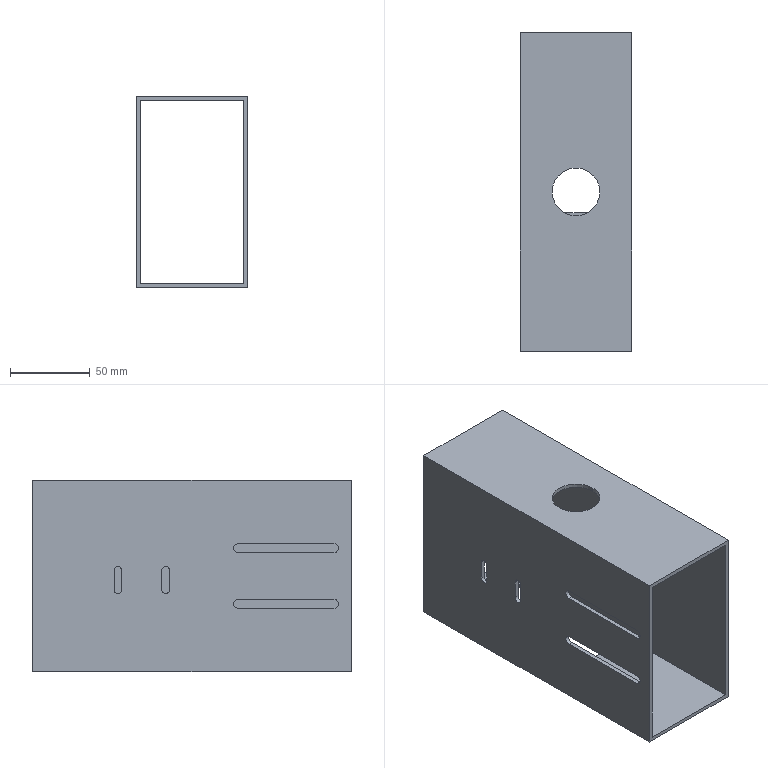Part | SolidWorks | features HoleWzd 2, Cut 1, Extrusion 1, ICE 1 | 1 solid | 34 faces | box 70 x 200 x 120 mm | volume 169957 mm3 | plane 22 | cylinder 12 | commonest cylinder face diameters 4.8 x6 5.8 x4 30 x2
STEP:
#1=CARTESIAN_POINT('',(2.5,48.9,-56.5));
#2=VERTEX_POINT('',#1);
#3=CARTESIAN_POINT('',(2.5,46.5,-54.1));
#4=VERTEX_POINT('',#3);
#5=CARTESIAN_POINT('',(2.5,46.5,-56.5));
#6=DIRECTION('',(1.,0.,0.));
#7=DIRECTION('',(0.,0.,-1.));
#8=AXIS2_PLACEMENT_3D('',#5,#6,#7);
#9=CIRCLE('',#8,2.4);
#10=EDGE_CURVE('',#2,#4,#9,.T.);
#11=ORIENTED_EDGE('',*,*,#10,.T.);
#12=CARTESIAN_POINT('',(0.,46.5,-54.1));
#13=VERTEX_POINT('',#12);
#14=CARTESIAN_POINT('',(0.,46.5,-54.1));
#15=DIRECTION('',(-1.,0.,0.));
#16=VECTOR('',#15,1000.);
#17=LINE('',#14,#16);
#18=EDGE_CURVE('',#4,#13,#17,.T.);
#19=ORIENTED_EDGE('',*,*,#18,.T.);
#20=CARTESIAN_POINT('',(0.,48.9,-56.5));
#21=VERTEX_POINT('',#20);
#22=CARTESIAN_POINT('',(0.,46.5,-56.5));
#23=DIRECTION('',(-1.,0.,0.));
#24=DIRECTION('',(0.,0.,1.));
#25=AXIS2_PLACEMENT_3D('',#22,#23,#24);
#26=CIRCLE('',#25,2.4);
#27=EDGE_CURVE('',#13,#21,#26,.T.);
#28=ORIENTED_EDGE('',*,*,#27,.T.);
#29=CARTESIAN_POINT('',(2.501,48.9,-56.5));
#30=DIRECTION('',(1.,0.,0.));
#31=VECTOR('',#30,1000.);
#32=LINE('',#29,#31);
#33=EDGE_CURVE('',#21,#2,#32,.T.);
#34=ORIENTED_EDGE('',*,*,#33,.T.);
#35=EDGE_LOOP('',(#11,#19,#28,#34));
#36=FACE_OUTER_BOUND('',#35,.T.);
#37=CARTESIAN_POINT('',(0.,46.5,-56.5));
#38=DIRECTION('',(-1.,0.,0.));
#39=DIRECTION('',(0.,0.,1.));
#40=AXIS2_PLACEMENT_3D('',#37,#38,#39);
#41=CYLINDRICAL_SURFACE('',#40,2.4);
#42=ADVANCED_FACE('',(#36),#41,.F.);
#43=CARTESIAN_POINT('',(2.5,18.9,-56.5));
#44=VERTEX_POINT('',#43);
#45=CARTESIAN_POINT('',(2.5,16.5,-54.1));
#46=VERTEX_POINT('',#45);
#47=CARTESIAN_POINT('',(2.5,16.5,-56.5));
#48=DIRECTION('',(1.,0.,0.));
#49=DIRECTION('',(0.,0.,-1.));
#50=AXIS2_PLACEMENT_3D('',#47,#48,#49);
#51=CIRCLE('',#50,2.4);
#52=EDGE_CURVE('',#44,#46,#51,.T.);
#53=ORIENTED_EDGE('',*,*,#52,.T.);
#54=CARTESIAN_POINT('',(0.,16.5,-54.1));
#55=VERTEX_POINT('',#54);
#56=CARTESIAN_POINT('',(0.,16.5,-54.1));
#57=DIRECTION('',(-1.,0.,0.));
#58=VECTOR('',#57,1000.);
#59=LINE('',#56,#58);
#60=EDGE_CURVE('',#46,#55,#59,.T.);
#61=ORIENTED_EDGE('',*,*,#60,.T.);
#62=CARTESIAN_POINT('',(0.,18.9,-56.5));
#63=VERTEX_POINT('',#62);
#64=CARTESIAN_POINT('',(0.,16.5,-56.5));
#65=DIRECTION('',(-1.,0.,0.));
#66=DIRECTION('',(0.,0.,1.));
#67=AXIS2_PLACEMENT_3D('',#64,#65,#66);
#68=CIRCLE('',#67,2.4);
#69=EDGE_CURVE('',#55,#63,#68,.T.);
#70=ORIENTED_EDGE('',*,*,#69,.T.);
#71=CARTESIAN_POINT('',(2.501,18.9,-56.5));
#72=DIRECTION('',(1.,0.,0.));
#73=VECTOR('',#72,1000.);
#74=LINE('',#71,#73);
#75=EDGE_CURVE('',#63,#44,#74,.T.);
#76=ORIENTED_EDGE('',*,*,#75,.T.);
#77=EDGE_LOOP('',(#53,#61,#70,#76));
#78=FACE_OUTER_BOUND('',#77,.T.);
#79=CARTESIAN_POINT('',(0.,16.5,-56.5));
#80=DIRECTION('',(-1.,0.,0.));
#81=DIRECTION('',(0.,0.,1.));
#82=AXIS2_PLACEMENT_3D('',#79,#80,#81);
#83=CYLINDRICAL_SURFACE('',#82,2.4);
#84=ADVANCED_FACE('',(#78),#83,.F.);
#85=CARTESIAN_POINT('',(20.,0.,-2.5));
#86=VERTEX_POINT('',#85);
#87=CARTESIAN_POINT('',(50.,0.,-2.5));
#88=VERTEX_POINT('',#87);
#89=CARTESIAN_POINT('',(35.,0.,-2.5));
#90=DIRECTION('',(0.,0.,1.));
#91=DIRECTION('',(-1.,0.,0.));
#92=AXIS2_PLACEMENT_3D('',#89,#90,#91);
#93=CIRCLE('',#92,15.);
#94=EDGE_CURVE('',#86,#88,#93,.T.);
#95=ORIENTED_EDGE('',*,*,#94,.F.);
#96=CARTESIAN_POINT('',(20.,0.,0.));
#97=VERTEX_POINT('',#96);
#98=CARTESIAN_POINT('',(20.,0.,-120.001));
#99=DIRECTION('',(0.,0.,1.));
#100=VECTOR('',#99,1000.);
#101=LINE('',#98,#100);
#102=EDGE_CURVE('',#86,#97,#101,.T.);
#103=ORIENTED_EDGE('',*,*,#102,.T.);
#104=CARTESIAN_POINT('',(50.,0.,0.));
#105=VERTEX_POINT('',#104);
#106=CARTESIAN_POINT('',(35.,0.,0.));
#107=DIRECTION('',(0.,0.,1.));
#108=DIRECTION('',(1.,0.,0.));
#109=AXIS2_PLACEMENT_3D('',#106,#107,#108);
#110=CIRCLE('',#109,15.);
#111=EDGE_CURVE('',#97,#105,#110,.T.);
#112=ORIENTED_EDGE('',*,*,#111,.T.);
#113=CARTESIAN_POINT('',(50.,0.,-120.001));
#114=DIRECTION('',(0.,0.,1.));
#115=VECTOR('',#114,1000.);
#116=LINE('',#113,#115);
#117=EDGE_CURVE('',#88,#105,#116,.T.);
#118=ORIENTED_EDGE('',*,*,#117,.F.);
#119=EDGE_LOOP('',(#95,#103,#112,#118));
#120=FACE_OUTER_BOUND('',#119,.T.);
#121=CARTESIAN_POINT('',(35.,0.,-120.001));
#122=DIRECTION('',(0.,0.,1.));
#123=DIRECTION('',(1.,0.,0.));
#124=AXIS2_PLACEMENT_3D('',#121,#122,#123);
#125=CYLINDRICAL_SURFACE('',#124,15.);
#126=ADVANCED_FACE('',(#120),#125,.F.);
#127=CARTESIAN_POINT('',(0.,-89.,-39.6));
#128=VERTEX_POINT('',#127);
#129=CARTESIAN_POINT('',(0.,-29.,-39.6));
#130=VERTEX_POINT('',#129);
#131=CARTESIAN_POINT('',(0.,-89.,-39.6));
#132=DIRECTION('',(0.,1.,0.));
#133=VECTOR('',#132,1000.);
#134=LINE('',#131,#133);
#135=EDGE_CURVE('',#128,#130,#134,.T.);
#136=ORIENTED_EDGE('',*,*,#135,.F.);
#137=CARTESIAN_POINT('',(0.,-89.,-45.4));
#138=VERTEX_POINT('',#137);
#139=CARTESIAN_POINT('',(0.,-89.,-42.5));
#140=DIRECTION('',(-1.,0.,0.));
#141=DIRECTION('',(0.,0.,1.));
#142=AXIS2_PLACEMENT_3D('',#139,#140,#141);
#143=CIRCLE('',#142,2.9);
#144=EDGE_CURVE('',#138,#128,#143,.T.);
#145=ORIENTED_EDGE('',*,*,#144,.F.);
#146=CARTESIAN_POINT('',(0.,-29.,-45.4));
#147=VERTEX_POINT('',#146);
#148=CARTESIAN_POINT('',(0.,-89.,-45.4));
#149=DIRECTION('',(0.,1.,0.));
#150=VECTOR('',#149,1000.);
#151=LINE('',#148,#150);
#152=EDGE_CURVE('',#138,#147,#151,.T.);
#153=ORIENTED_EDGE('',*,*,#152,.T.);
#154=CARTESIAN_POINT('',(0.,-29.,-42.5));
#155=DIRECTION('',(-1.,0.,0.));
#156=DIRECTION('',(0.,0.,1.));
#157=AXIS2_PLACEMENT_3D('',#154,#155,#156);
#158=CIRCLE('',#157,2.9);
#159=EDGE_CURVE('',#130,#147,#158,.T.);
#160=ORIENTED_EDGE('',*,*,#159,.F.);
#161=EDGE_LOOP('',(#136,#145,#153,#160));
#162=FACE_BOUND('',#161,.T.);
#163=CARTESIAN_POINT('',(0.,48.9,-68.5));
#164=VERTEX_POINT('',#163);
#165=CARTESIAN_POINT('',(0.,48.9,-68.5));
#166=DIRECTION('',(0.,0.,1.));
#167=VECTOR('',#166,1000.);
#168=LINE('',#165,#167);
#169=EDGE_CURVE('',#164,#21,#168,.T.);
#170=ORIENTED_EDGE('',*,*,#169,.T.);
#171=ORIENTED_EDGE('',*,*,#27,.F.);
#172=CARTESIAN_POINT('',(0.,44.1,-56.5));
#173=VERTEX_POINT('',#172);
#174=CARTESIAN_POINT('',(0.,46.5,-56.5));
#175=DIRECTION('',(-1.,0.,0.));
#176=DIRECTION('',(0.,0.,1.));
#177=AXIS2_PLACEMENT_3D('',#174,#175,#176);
#178=CIRCLE('',#177,2.4);
#179=EDGE_CURVE('',#173,#13,#178,.T.);
#180=ORIENTED_EDGE('',*,*,#179,.F.);
#181=CARTESIAN_POINT('',(0.,44.1,-68.5));
#182=VERTEX_POINT('',#181);
#183=CARTESIAN_POINT('',(0.,44.1,-68.5));
#184=DIRECTION('',(0.,0.,1.));
#185=VECTOR('',#184,1000.);
#186=LINE('',#183,#185);
#187=EDGE_CURVE('',#182,#173,#186,.T.);
#188=ORIENTED_EDGE('',*,*,#187,.F.);
#189=CARTESIAN_POINT('',(0.,46.5,-68.5));
#190=DIRECTION('',(-1.,0.,0.));
#191=DIRECTION('',(0.,0.,1.));
#192=AXIS2_PLACEMENT_3D('',#189,#190,#191);
#193=CIRCLE('',#192,2.4);
#194=EDGE_CURVE('',#164,#182,#193,.T.);
#195=ORIENTED_EDGE('',*,*,#194,.F.);
#196=EDGE_LOOP('',(#170,#171,#180,#188,#195));
#197=FACE_BOUND('',#196,.T.);
#198=CARTESIAN_POINT('',(0.,-100.,-120.));
#199=VERTEX_POINT('',#198);
#200=CARTESIAN_POINT('',(0.,-100.,0.));
#201=VERTEX_POINT('',#200);
#202=CARTESIAN_POINT('',(0.,-100.,0.));
#203=DIRECTION('',(0.,0.,1.));
#204=VECTOR('',#203,1000.);
#205=LINE('',#202,#204);
#206=EDGE_CURVE('',#199,#201,#205,.T.);
#207=ORIENTED_EDGE('',*,*,#206,.T.);
#208=CARTESIAN_POINT('',(0.,100.,0.));
#209=VERTEX_POINT('',#208);
#210=CARTESIAN_POINT('',(0.,100.,0.));
#211=DIRECTION('',(0.,-1.,0.));
#212=VECTOR('',#211,1000.);
#213=LINE('',#210,#212);
#214=EDGE_CURVE('',#209,#201,#213,.T.);
#215=ORIENTED_EDGE('',*,*,#214,.F.);
#216=CARTESIAN_POINT('',(0.,100.,-120.));
#217=VERTEX_POINT('',#216);
#218=CARTESIAN_POINT('',(0.,100.,0.));
#219=DIRECTION('',(0.,0.,1.));
#220=VECTOR('',#219,1000.);
#221=LINE('',#218,#220);
#222=EDGE_CURVE('',#217,#209,#221,.T.);
#223=ORIENTED_EDGE('',*,*,#222,.F.);
#224=CARTESIAN_POINT('',(0.,100.,-120.));
#225=DIRECTION('',(0.,-1.,0.));
#226=VECTOR('',#225,1000.);
#227=LINE('',#224,#226);
#228=EDGE_CURVE('',#217,#199,#227,.T.);
#229=ORIENTED_EDGE('',*,*,#228,.T.);
#230=EDGE_LOOP('',(#207,#215,#223,#229));
#231=FACE_OUTER_BOUND('',#230,.T.);
#232=CARTESIAN_POINT('',(0.,14.1,-56.5));
#233=VERTEX_POINT('',#232);
#234=CARTESIAN_POINT('',(0.,16.5,-56.5));
#235=DIRECTION('',(-1.,0.,0.));
#236=DIRECTION('',(0.,0.,1.));
#237=AXIS2_PLACEMENT_3D('',#234,#235,#236);
#238=CIRCLE('',#237,2.4);
#239=EDGE_CURVE('',#233,#55,#238,.T.);
#240=ORIENTED_EDGE('',*,*,#239,.F.);
#241=CARTESIAN_POINT('',(0.,14.1,-68.5));
#242=VERTEX_POINT('',#241);
#243=CARTESIAN_POINT('',(0.,14.1,-68.5));
#244=DIRECTION('',(0.,0.,1.));
#245=VECTOR('',#244,1000.);
#246=LINE('',#243,#245);
#247=EDGE_CURVE('',#242,#233,#246,.T.);
#248=ORIENTED_EDGE('',*,*,#247,.F.);
#249=CARTESIAN_POINT('',(0.,18.9,-68.5));
#250=VERTEX_POINT('',#249);
#251=CARTESIAN_POINT('',(0.,16.5,-68.5));
#252=DIRECTION('',(-1.,0.,0.));
#253=DIRECTION('',(0.,0.,1.));
#254=AXIS2_PLACEMENT_3D('',#251,#252,#253);
#255=CIRCLE('',#254,2.4);
#256=EDGE_CURVE('',#250,#242,#255,.T.);
#257=ORIENTED_EDGE('',*,*,#256,.F.);
#258=CARTESIAN_POINT('',(0.,18.9,-68.5));
#259=DIRECTION('',(0.,0.,1.));
#260=VECTOR('',#259,1000.);
#261=LINE('',#258,#260);
#262=EDGE_CURVE('',#250,#63,#261,.T.);
#263=ORIENTED_EDGE('',*,*,#262,.T.);
#264=ORIENTED_EDGE('',*,*,#69,.F.);
#265=EDGE_LOOP('',(#240,#248,#257,#263,#264));
#266=FACE_BOUND('',#265,.T.);
#267=CARTESIAN_POINT('',(0.,-89.,-74.6));
#268=VERTEX_POINT('',#267);
#269=CARTESIAN_POINT('',(0.,-29.,-74.6));
#270=VERTEX_POINT('',#269);
#271=CARTESIAN_POINT('',(0.,-89.,-74.6));
#272=DIRECTION('',(0.,1.,0.));
#273=VECTOR('',#272,1000.);
#274=LINE('',#271,#273);
#275=EDGE_CURVE('',#268,#270,#274,.T.);
#276=ORIENTED_EDGE('',*,*,#275,.F.);
#277=CARTESIAN_POINT('',(0.,-89.,-80.4));
#278=VERTEX_POINT('',#277);
#279=CARTESIAN_POINT('',(0.,-89.,-77.5));
#280=DIRECTION('',(-1.,0.,0.));
#281=DIRECTION('',(0.,0.,1.));
#282=AXIS2_PLACEMENT_3D('',#279,#280,#281);
#283=CIRCLE('',#282,2.9);
#284=EDGE_CURVE('',#278,#268,#283,.T.);
#285=ORIENTED_EDGE('',*,*,#284,.F.);
#286=CARTESIAN_POINT('',(0.,-29.,-80.4));
#287=VERTEX_POINT('',#286);
#288=CARTESIAN_POINT('',(0.,-89.,-80.4));
#289=DIRECTION('',(0.,1.,0.));
#290=VECTOR('',#289,1000.);
#291=LINE('',#288,#290);
#292=EDGE_CURVE('',#278,#287,#291,.T.);
#293=ORIENTED_EDGE('',*,*,#292,.T.);
#294=CARTESIAN_POINT('',(0.,-29.,-77.5));
#295=DIRECTION('',(-1.,0.,0.));
#296=DIRECTION('',(0.,0.,1.));
#297=AXIS2_PLACEMENT_3D('',#294,#295,#296);
#298=CIRCLE('',#297,2.9);
#299=EDGE_CURVE('',#270,#287,#298,.T.);
#300=ORIENTED_EDGE('',*,*,#299,.F.);
#301=EDGE_LOOP('',(#276,#285,#293,#300));
#302=FACE_BOUND('',#301,.T.);
#303=CARTESIAN_POINT('',(0.,100.,0.));
#304=DIRECTION('',(1.,0.,0.));
#305=DIRECTION('',(0.,0.,-1.));
#306=AXIS2_PLACEMENT_3D('',#303,#304,#305);
#307=PLANE('',#306);
#308=ADVANCED_FACE('',(#162,#197,#231,#266,#302),#307,.F.);
#309=CARTESIAN_POINT('',(2.5,-89.,-80.4));
#310=VERTEX_POINT('',#309);
#311=CARTESIAN_POINT('',(2.5,-29.,-80.4));
#312=VERTEX_POINT('',#311);
#313=CARTESIAN_POINT('',(2.5,100.,-80.4));
#314=DIRECTION('',(0.,1.,0.));
#315=VECTOR('',#314,1000.);
#316=LINE('',#313,#315);
#317=EDGE_CURVE('',#310,#312,#316,.T.);
#318=ORIENTED_EDGE('',*,*,#317,.F.);
#319=CARTESIAN_POINT('',(2.5,-89.,-74.6));
#320=VERTEX_POINT('',#319);
#321=CARTESIAN_POINT('',(2.5,-89.,-77.5));
#322=DIRECTION('',(1.,0.,0.));
#323=DIRECTION('',(0.,0.,-1.));
#324=AXIS2_PLACEMENT_3D('',#321,#322,#323);
#325=CIRCLE('',#324,2.9);
#326=EDGE_CURVE('',#320,#310,#325,.T.);
#327=ORIENTED_EDGE('',*,*,#326,.F.);
#328=CARTESIAN_POINT('',(2.5,-29.,-74.6));
#329=VERTEX_POINT('',#328);
#330=CARTESIAN_POINT('',(2.5,100.,-74.6));
#331=DIRECTION('',(0.,-1.,0.));
#332=VECTOR('',#331,1000.);
#333=LINE('',#330,#332);
#334=EDGE_CURVE('',#329,#320,#333,.T.);
#335=ORIENTED_EDGE('',*,*,#334,.F.);
#336=CARTESIAN_POINT('',(2.5,-29.,-77.5));
#337=DIRECTION('',(1.,0.,0.));
#338=DIRECTION('',(0.,0.,-1.));
#339=AXIS2_PLACEMENT_3D('',#336,#337,#338);
#340=CIRCLE('',#339,2.9);
#341=EDGE_CURVE('',#312,#329,#340,.T.);
#342=ORIENTED_EDGE('',*,*,#341,.F.);
#343=EDGE_LOOP('',(#318,#327,#335,#342));
#344=FACE_BOUND('',#343,.T.);
#345=CARTESIAN_POINT('',(2.5,-89.,-45.4));
#346=VERTEX_POINT('',#345);
#347=CARTESIAN_POINT('',(2.5,-29.,-45.4));
#348=VERTEX_POINT('',#347);
#349=CARTESIAN_POINT('',(2.5,100.,-45.4));
#350=DIRECTION('',(0.,1.,0.));
#351=VECTOR('',#350,1000.);
#352=LINE('',#349,#351);
#353=EDGE_CURVE('',#346,#348,#352,.T.);
#354=ORIENTED_EDGE('',*,*,#353,.F.);
#355=CARTESIAN_POINT('',(2.5,-89.,-39.6));
#356=VERTEX_POINT('',#355);
#357=CARTESIAN_POINT('',(2.5,-89.,-42.5));
#358=DIRECTION('',(1.,0.,0.));
#359=DIRECTION('',(0.,0.,-1.));
#360=AXIS2_PLACEMENT_3D('',#357,#358,#359);
#361=CIRCLE('',#360,2.9);
#362=EDGE_CURVE('',#356,#346,#361,.T.);
#363=ORIENTED_EDGE('',*,*,#362,.F.);
#364=CARTESIAN_POINT('',(2.5,-29.,-39.6));
#365=VERTEX_POINT('',#364);
#366=CARTESIAN_POINT('',(2.5,100.,-39.6));
#367=DIRECTION('',(0.,-1.,0.));
#368=VECTOR('',#367,1000.);
#369=LINE('',#366,#368);
#370=EDGE_CURVE('',#365,#356,#369,.T.);
#371=ORIENTED_EDGE('',*,*,#370,.F.);
#372=CARTESIAN_POINT('',(2.5,-29.,-42.5));
#373=DIRECTION('',(1.,0.,0.));
#374=DIRECTION('',(0.,0.,-1.));
#375=AXIS2_PLACEMENT_3D('',#372,#373,#374);
#376=CIRCLE('',#375,2.9);
#377=EDGE_CURVE('',#348,#365,#376,.T.);
#378=ORIENTED_EDGE('',*,*,#377,.F.);
#379=EDGE_LOOP('',(#354,#363,#371,#378));
#380=FACE_BOUND('',#379,.T.);
#381=CARTESIAN_POINT('',(2.5,-100.,-117.5));
#382=VERTEX_POINT('',#381);
#383=CARTESIAN_POINT('',(2.5,-100.,-2.5));
#384=VERTEX_POINT('',#383);
#385=CARTESIAN_POINT('',(2.5,-100.,-2.5));
#386=DIRECTION('',(0.,0.,1.));
#387=VECTOR('',#386,1000.);
#388=LINE('',#385,#387);
#389=EDGE_CURVE('',#382,#384,#388,.T.);
#390=ORIENTED_EDGE('',*,*,#389,.F.);
#391=CARTESIAN_POINT('',(2.5,100.,-117.5));
#392=VERTEX_POINT('',#391);
#393=CARTESIAN_POINT('',(2.5,100.,-117.5));
#394=DIRECTION('',(0.,-1.,0.));
#395=VECTOR('',#394,1000.);
#396=LINE('',#393,#395);
#397=EDGE_CURVE('',#392,#382,#396,.T.);
#398=ORIENTED_EDGE('',*,*,#397,.F.);
#399=CARTESIAN_POINT('',(2.5,100.,-2.5));
#400=VERTEX_POINT('',#399);
#401=CARTESIAN_POINT('',(2.5,100.,-2.5));
#402=DIRECTION('',(0.,0.,1.));
#403=VECTOR('',#402,1000.);
#404=LINE('',#401,#403);
#405=EDGE_CURVE('',#392,#400,#404,.T.);
#406=ORIENTED_EDGE('',*,*,#405,.T.);
#407=CARTESIAN_POINT('',(2.5,100.,-2.5));
#408=DIRECTION('',(0.,-1.,0.));
#409=VECTOR('',#408,1000.);
#410=LINE('',#407,#409);
#411=EDGE_CURVE('',#400,#384,#410,.T.);
#412=ORIENTED_EDGE('',*,*,#411,.T.);
#413=EDGE_LOOP('',(#390,#398,#406,#412));
#414=FACE_OUTER_BOUND('',#413,.T.);
#415=ORIENTED_EDGE('',*,*,#52,.F.);
#416=CARTESIAN_POINT('',(2.5,18.9,-68.5));
#417=VERTEX_POINT('',#416);
#418=CARTESIAN_POINT('',(2.5,18.9,-2.5));
#419=DIRECTION('',(0.,0.,-1.));
#420=VECTOR('',#419,1000.);
#421=LINE('',#418,#420);
#422=EDGE_CURVE('',#44,#417,#421,.T.);
#423=ORIENTED_EDGE('',*,*,#422,.T.);
#424=CARTESIAN_POINT('',(2.5,14.1,-68.5));
#425=VERTEX_POINT('',#424);
#426=CARTESIAN_POINT('',(2.5,16.5,-68.5));
#427=DIRECTION('',(1.,0.,0.));
#428=DIRECTION('',(0.,0.,-1.));
#429=AXIS2_PLACEMENT_3D('',#426,#427,#428);
#430=CIRCLE('',#429,2.4);
#431=EDGE_CURVE('',#425,#417,#430,.T.);
#432=ORIENTED_EDGE('',*,*,#431,.F.);
#433=CARTESIAN_POINT('',(2.5,14.1,-56.5));
#434=VERTEX_POINT('',#433);
#435=CARTESIAN_POINT('',(2.5,14.1,-2.5));
#436=DIRECTION('',(0.,0.,-1.));
#437=VECTOR('',#436,1000.);
#438=LINE('',#435,#437);
#439=EDGE_CURVE('',#434,#425,#438,.T.);
#440=ORIENTED_EDGE('',*,*,#439,.F.);
#441=CARTESIAN_POINT('',(2.5,16.5,-56.5));
#442=DIRECTION('',(1.,0.,0.));
#443=DIRECTION('',(0.,0.,-1.));
#444=AXIS2_PLACEMENT_3D('',#441,#442,#443);
#445=CIRCLE('',#444,2.4);
#446=EDGE_CURVE('',#46,#434,#445,.T.);
#447=ORIENTED_EDGE('',*,*,#446,.F.);
#448=EDGE_LOOP('',(#415,#423,#432,#440,#447));
#449=FACE_BOUND('',#448,.T.);
#450=ORIENTED_EDGE('',*,*,#10,.F.);
#451=CARTESIAN_POINT('',(2.5,48.9,-68.5));
#452=VERTEX_POINT('',#451);
#453=CARTESIAN_POINT('',(2.5,48.9,-2.5));
#454=DIRECTION('',(0.,0.,-1.));
#455=VECTOR('',#454,1000.);
#456=LINE('',#453,#455);
#457=EDGE_CURVE('',#2,#452,#456,.T.);
#458=ORIENTED_EDGE('',*,*,#457,.T.);
#459=CARTESIAN_POINT('',(2.5,44.1,-68.5));
#460=VERTEX_POINT('',#459);
#461=CARTESIAN_POINT('',(2.5,46.5,-68.5));
#462=DIRECTION('',(1.,0.,0.));
#463=DIRECTION('',(0.,0.,-1.));
#464=AXIS2_PLACEMENT_3D('',#461,#462,#463);
#465=CIRCLE('',#464,2.4);
#466=EDGE_CURVE('',#460,#452,#465,.T.);
#467=ORIENTED_EDGE('',*,*,#466,.F.);
#468=CARTESIAN_POINT('',(2.5,44.1,-56.5));
#469=VERTEX_POINT('',#468);
#470=CARTESIAN_POINT('',(2.5,44.1,-2.5));
#471=DIRECTION('',(0.,0.,-1.));
#472=VECTOR('',#471,1000.);
#473=LINE('',#470,#472);
#474=EDGE_CURVE('',#469,#460,#473,.T.);
#475=ORIENTED_EDGE('',*,*,#474,.F.);
#476=CARTESIAN_POINT('',(2.5,46.5,-56.5));
#477=DIRECTION('',(1.,0.,0.));
#478=DIRECTION('',(0.,0.,-1.));
#479=AXIS2_PLACEMENT_3D('',#476,#477,#478);
#480=CIRCLE('',#479,2.4);
#481=EDGE_CURVE('',#4,#469,#480,.T.);
#482=ORIENTED_EDGE('',*,*,#481,.F.);
#483=EDGE_LOOP('',(#450,#458,#467,#475,#482));
#484=FACE_BOUND('',#483,.T.);
#485=CARTESIAN_POINT('',(2.5,100.,-2.5));
#486=DIRECTION('',(1.,0.,0.));
#487=DIRECTION('',(0.,0.,-1.));
#488=AXIS2_PLACEMENT_3D('',#485,#486,#487);
#489=PLANE('',#488);
#490=ADVANCED_FACE('',(#344,#380,#414,#449,#484),#489,.T.);
#491=ORIENTED_EDGE('',*,*,#222,.T.);
#492=CARTESIAN_POINT('',(70.,100.,0.));
#493=VERTEX_POINT('',#492);
#494=CARTESIAN_POINT('',(0.,100.,0.));
#495=DIRECTION('',(1.,0.,0.));
#496=VECTOR('',#495,1000.);
#497=LINE('',#494,#496);
#498=EDGE_CURVE('',#209,#493,#497,.T.);
#499=ORIENTED_EDGE('',*,*,#498,.T.);
#500=CARTESIAN_POINT('',(70.,100.,-120.));
#501=VERTEX_POINT('',#500);
#502=CARTESIAN_POINT('',(70.,100.,0.));
#503=DIRECTION('',(0.,0.,-1.));
#504=VECTOR('',#503,1000.);
#505=LINE('',#502,#504);
#506=EDGE_CURVE('',#493,#501,#505,.T.);
#507=ORIENTED_EDGE('',*,*,#506,.T.);
#508=CARTESIAN_POINT('',(0.,100.,-120.));
#509=DIRECTION('',(-1.,0.,0.));
#510=VECTOR('',#509,1000.);
#511=LINE('',#508,#510);
#512=EDGE_CURVE('',#501,#217,#511,.T.);
#513=ORIENTED_EDGE('',*,*,#512,.T.);
#514=EDGE_LOOP('',(#491,#499,#507,#513));
#515=FACE_OUTER_BOUND('',#514,.T.);
#516=ORIENTED_EDGE('',*,*,#405,.F.);
#517=CARTESIAN_POINT('',(67.5,100.,-117.5));
#518=VERTEX_POINT('',#517);
#519=CARTESIAN_POINT('',(2.5,100.,-117.5));
#520=DIRECTION('',(-1.,0.,0.));
#521=VECTOR('',#520,1000.);
#522=LINE('',#519,#521);
#523=EDGE_CURVE('',#518,#392,#522,.T.);
#524=ORIENTED_EDGE('',*,*,#523,.F.);
#525=CARTESIAN_POINT('',(67.5,100.,-2.5));
#526=VERTEX_POINT('',#525);
#527=CARTESIAN_POINT('',(67.5,100.,-2.5));
#528=DIRECTION('',(0.,0.,-1.));
#529=VECTOR('',#528,1000.);
#530=LINE('',#527,#529);
#531=EDGE_CURVE('',#526,#518,#530,.T.);
#532=ORIENTED_EDGE('',*,*,#531,.F.);
#533=CARTESIAN_POINT('',(2.5,100.,-2.5));
#534=DIRECTION('',(1.,0.,0.));
#535=VECTOR('',#534,1000.);
#536=LINE('',#533,#535);
#537=EDGE_CURVE('',#400,#526,#536,.T.);
#538=ORIENTED_EDGE('',*,*,#537,.F.);
#539=EDGE_LOOP('',(#516,#524,#532,#538));
#540=FACE_BOUND('',#539,.T.);
#541=CARTESIAN_POINT('',(0.,100.,0.));
#542=DIRECTION('',(0.,-1.,0.));
#543=DIRECTION('',(0.,0.,-1.));
#544=AXIS2_PLACEMENT_3D('',#541,#542,#543);
#545=PLANE('',#544);
#546=ADVANCED_FACE('',(#515,#540),#545,.F.);
#547=ORIENTED_EDGE('',*,*,#206,.F.);
#548=CARTESIAN_POINT('',(70.,-100.,-120.));
#549=VERTEX_POINT('',#548);
#550=CARTESIAN_POINT('',(0.,-100.,-120.));
#551=DIRECTION('',(-1.,0.,0.));
#552=VECTOR('',#551,1000.);
#553=LINE('',#550,#552);
#554=EDGE_CURVE('',#549,#199,#553,.T.);
#555=ORIENTED_EDGE('',*,*,#554,.F.);
#556=CARTESIAN_POINT('',(70.,-100.,0.));
#557=VERTEX_POINT('',#556);
#558=CARTESIAN_POINT('',(70.,-100.,0.));
#559=DIRECTION('',(0.,0.,-1.));
#560=VECTOR('',#559,1000.);
#561=LINE('',#558,#560);
#562=EDGE_CURVE('',#557,#549,#561,.T.);
#563=ORIENTED_EDGE('',*,*,#562,.F.);
#564=CARTESIAN_POINT('',(0.,-100.,0.));
#565=DIRECTION('',(1.,0.,0.));
#566=VECTOR('',#565,1000.);
#567=LINE('',#564,#566);
#568=EDGE_CURVE('',#201,#557,#567,.T.);
#569=ORIENTED_EDGE('',*,*,#568,.F.);
#570=EDGE_LOOP('',(#547,#555,#563,#569));
#571=FACE_OUTER_BOUND('',#570,.T.);
#572=CARTESIAN_POINT('',(67.5,-100.,-117.5));
#573=VERTEX_POINT('',#572);
#574=CARTESIAN_POINT('',(2.5,-100.,-117.5));
#575=DIRECTION('',(-1.,0.,0.));
#576=VECTOR('',#575,1000.);
#577=LINE('',#574,#576);
#578=EDGE_CURVE('',#573,#382,#577,.T.);
#579=ORIENTED_EDGE('',*,*,#578,.T.);
#580=ORIENTED_EDGE('',*,*,#389,.T.);
#581=CARTESIAN_POINT('',(67.5,-100.,-2.5));
#582=VERTEX_POINT('',#581);
#583=CARTESIAN_POINT('',(2.5,-100.,-2.5));
#584=DIRECTION('',(1.,0.,0.));
#585=VECTOR('',#584,1000.);
#586=LINE('',#583,#585);
#587=EDGE_CURVE('',#384,#582,#586,.T.);
#588=ORIENTED_EDGE('',*,*,#587,.T.);
#589=CARTESIAN_POINT('',(67.5,-100.,-2.5));
#590=DIRECTION('',(0.,0.,-1.));
#591=VECTOR('',#590,1000.);
#592=LINE('',#589,#591);
#593=EDGE_CURVE('',#582,#573,#592,.T.);
#594=ORIENTED_EDGE('',*,*,#593,.T.);
#595=EDGE_LOOP('',(#579,#580,#588,#594));
#596=FACE_BOUND('',#595,.T.);
#597=CARTESIAN_POINT('',(0.,-100.,0.));
#598=DIRECTION('',(0.,-1.,0.));
#599=DIRECTION('',(0.,0.,-1.));
#600=AXIS2_PLACEMENT_3D('',#597,#598,#599);
#601=PLANE('',#600);
#602=ADVANCED_FACE('',(#571,#596),#601,.T.);
#603=CARTESIAN_POINT('',(35.,0.,0.));
#604=DIRECTION('',(0.,0.,1.));
#605=DIRECTION('',(1.,0.,0.));
#606=AXIS2_PLACEMENT_3D('',#603,#604,#605);
#607=CIRCLE('',#606,15.);
#608=EDGE_CURVE('',#105,#97,#607,.T.);
#609=ORIENTED_EDGE('',*,*,#608,.F.);
#610=ORIENTED_EDGE('',*,*,#111,.F.);
#611=EDGE_LOOP('',(#609,#610));
#612=FACE_BOUND('',#611,.T.);
#613=ORIENTED_EDGE('',*,*,#568,.T.);
#614=CARTESIAN_POINT('',(70.,100.,0.));
#615=DIRECTION('',(0.,-1.,0.));
#616=VECTOR('',#615,1000.);
#617=LINE('',#614,#616);
#618=EDGE_CURVE('',#493,#557,#617,.T.);
#619=ORIENTED_EDGE('',*,*,#618,.F.);
#620=ORIENTED_EDGE('',*,*,#498,.F.);
#621=ORIENTED_EDGE('',*,*,#214,.T.);
#622=EDGE_LOOP('',(#613,#619,#620,#621));
#623=FACE_OUTER_BOUND('',#622,.T.);
#624=CARTESIAN_POINT('',(0.,100.,0.));
#625=DIRECTION('',(0.,0.,-1.));
#626=DIRECTION('',(-1.,0.,0.));
#627=AXIS2_PLACEMENT_3D('',#624,#625,#626);
#628=PLANE('',#627);
#629=ADVANCED_FACE('',(#612,#623),#628,.F.);
#630=ORIENTED_EDGE('',*,*,#562,.T.);
#631=CARTESIAN_POINT('',(70.,100.,-120.));
#632=DIRECTION('',(0.,-1.,0.));
#633=VECTOR('',#632,1000.);
#634=LINE('',#631,#633);
#635=EDGE_CURVE('',#501,#549,#634,.T.);
#636=ORIENTED_EDGE('',*,*,#635,.F.);
#637=ORIENTED_EDGE('',*,*,#506,.F.);
#638=ORIENTED_EDGE('',*,*,#618,.T.);
#639=EDGE_LOOP('',(#630,#636,#637,#638));
#640=FACE_OUTER_BOUND('',#639,.T.);
#641=CARTESIAN_POINT('',(70.,100.,0.));
#642=DIRECTION('',(-1.,0.,0.));
#643=DIRECTION('',(0.,0.,1.));
#644=AXIS2_PLACEMENT_3D('',#641,#642,#643);
#645=PLANE('',#644);
#646=ADVANCED_FACE('',(#640),#645,.F.);
#647=CARTESIAN_POINT('',(61.,85.,-120.));
#648=VERTEX_POINT('',#647);
#649=CARTESIAN_POINT('',(61.,-13.,-120.));
#650=VERTEX_POINT('',#649);
#651=CARTESIAN_POINT('',(61.,-13.,-120.));
#652=DIRECTION('',(0.,-1.,0.));
#653=VECTOR('',#652,1000.);
#654=LINE('',#651,#653);
#655=EDGE_CURVE('',#648,#650,#654,.T.);
#656=ORIENTED_EDGE('',*,*,#655,.F.);
#657=CARTESIAN_POINT('',(16.,85.,-120.));
#658=VERTEX_POINT('',#657);
#659=CARTESIAN_POINT('',(61.,85.,-120.));
#660=DIRECTION('',(1.,0.,0.));
#661=VECTOR('',#660,1000.);
#662=LINE('',#659,#661);
#663=EDGE_CURVE('',#658,#648,#662,.T.);
#664=ORIENTED_EDGE('',*,*,#663,.F.);
#665=CARTESIAN_POINT('',(16.,-13.,-120.));
#666=VERTEX_POINT('',#665);
#667=CARTESIAN_POINT('',(16.,-13.,-120.));
#668=DIRECTION('',(0.,1.,0.));
#669=VECTOR('',#668,1000.);
#670=LINE('',#667,#669);
#671=EDGE_CURVE('',#666,#658,#670,.T.);
#672=ORIENTED_EDGE('',*,*,#671,.F.);
#673=CARTESIAN_POINT('',(61.,-13.,-120.));
#674=DIRECTION('',(-1.,0.,0.));
#675=VECTOR('',#674,1000.);
#676=LINE('',#673,#675);
#677=EDGE_CURVE('',#650,#666,#676,.T.);
#678=ORIENTED_EDGE('',*,*,#677,.F.);
#679=EDGE_LOOP('',(#656,#664,#672,#678));
#680=FACE_BOUND('',#679,.T.);
#681=ORIENTED_EDGE('',*,*,#554,.T.);
#682=ORIENTED_EDGE('',*,*,#228,.F.);
#683=ORIENTED_EDGE('',*,*,#512,.F.);
#684=ORIENTED_EDGE('',*,*,#635,.T.);
#685=EDGE_LOOP('',(#681,#682,#683,#684));
#686=FACE_OUTER_BOUND('',#685,.T.);
#687=CARTESIAN_POINT('',(0.,100.,-120.));
#688=DIRECTION('',(0.,0.,1.));
#689=DIRECTION('',(1.,0.,0.));
#690=AXIS2_PLACEMENT_3D('',#687,#688,#689);
#691=PLANE('',#690);
#692=ADVANCED_FACE('',(#680,#686),#691,.F.);
#693=CARTESIAN_POINT('',(35.,0.,-2.5));
#694=DIRECTION('',(0.,0.,1.));
#695=DIRECTION('',(-1.,0.,0.));
#696=AXIS2_PLACEMENT_3D('',#693,#694,#695);
#697=CIRCLE('',#696,15.);
#698=EDGE_CURVE('',#88,#86,#697,.T.);
#699=ORIENTED_EDGE('',*,*,#698,.T.);
#700=ORIENTED_EDGE('',*,*,#94,.T.);
#701=EDGE_LOOP('',(#699,#700));
#702=FACE_BOUND('',#701,.T.);
#703=ORIENTED_EDGE('',*,*,#587,.F.);
#704=ORIENTED_EDGE('',*,*,#411,.F.);
#705=ORIENTED_EDGE('',*,*,#537,.T.);
#706=CARTESIAN_POINT('',(67.5,100.,-2.5));
#707=DIRECTION('',(0.,-1.,0.));
#708=VECTOR('',#707,1000.);
#709=LINE('',#706,#708);
#710=EDGE_CURVE('',#526,#582,#709,.T.);
#711=ORIENTED_EDGE('',*,*,#710,.T.);
#712=EDGE_LOOP('',(#703,#704,#705,#711));
#713=FACE_OUTER_BOUND('',#712,.T.);
#714=CARTESIAN_POINT('',(2.5,100.,-2.5));
#715=DIRECTION('',(0.,0.,-1.));
#716=DIRECTION('',(-1.,0.,0.));
#717=AXIS2_PLACEMENT_3D('',#714,#715,#716);
#718=PLANE('',#717);
#719=ADVANCED_FACE('',(#702,#713),#718,.T.);
#720=ORIENTED_EDGE('',*,*,#593,.F.);
#721=ORIENTED_EDGE('',*,*,#710,.F.);
#722=ORIENTED_EDGE('',*,*,#531,.T.);
#723=CARTESIAN_POINT('',(67.5,100.,-117.5));
#724=DIRECTION('',(0.,-1.,0.));
#725=VECTOR('',#724,1000.);
#726=LINE('',#723,#725);
#727=EDGE_CURVE('',#518,#573,#726,.T.);
#728=ORIENTED_EDGE('',*,*,#727,.T.);
#729=EDGE_LOOP('',(#720,#721,#722,#728));
#730=FACE_OUTER_BOUND('',#729,.T.);
#731=CARTESIAN_POINT('',(67.5,100.,-2.5));
#732=DIRECTION('',(-1.,0.,0.));
#733=DIRECTION('',(0.,0.,1.));
#734=AXIS2_PLACEMENT_3D('',#731,#732,#733);
#735=PLANE('',#734);
#736=ADVANCED_FACE('',(#730),#735,.T.);
#737=CARTESIAN_POINT('',(16.,85.,-117.5));
#738=VERTEX_POINT('',#737);
#739=CARTESIAN_POINT('',(61.,85.,-117.5));
#740=VERTEX_POINT('',#739);
#741=CARTESIAN_POINT('',(61.,85.,-117.5));
#742=DIRECTION('',(1.,0.,0.));
#743=VECTOR('',#742,1000.);
#744=LINE('',#741,#743);
#745=EDGE_CURVE('',#738,#740,#744,.T.);
#746=ORIENTED_EDGE('',*,*,#745,.T.);
#747=CARTESIAN_POINT('',(61.,-13.,-117.5));
#748=VERTEX_POINT('',#747);
#749=CARTESIAN_POINT('',(61.,-13.,-117.5));
#750=DIRECTION('',(0.,-1.,0.));
#751=VECTOR('',#750,1000.);
#752=LINE('',#749,#751);
#753=EDGE_CURVE('',#740,#748,#752,.T.);
#754=ORIENTED_EDGE('',*,*,#753,.T.);
#755=CARTESIAN_POINT('',(16.,-13.,-117.5));
#756=VERTEX_POINT('',#755);
#757=CARTESIAN_POINT('',(61.,-13.,-117.5));
#758=DIRECTION('',(-1.,0.,0.));
#759=VECTOR('',#758,1000.);
#760=LINE('',#757,#759);
#761=EDGE_CURVE('',#748,#756,#760,.T.);
#762=ORIENTED_EDGE('',*,*,#761,.T.);
#763=CARTESIAN_POINT('',(16.,-13.,-117.5));
#764=DIRECTION('',(0.,1.,0.));
#765=VECTOR('',#764,1000.);
#766=LINE('',#763,#765);
#767=EDGE_CURVE('',#756,#738,#766,.T.);
#768=ORIENTED_EDGE('',*,*,#767,.T.);
#769=EDGE_LOOP('',(#746,#754,#762,#768));
#770=FACE_BOUND('',#769,.T.);
#771=ORIENTED_EDGE('',*,*,#578,.F.);
#772=ORIENTED_EDGE('',*,*,#727,.F.);
#773=ORIENTED_EDGE('',*,*,#523,.T.);
#774=ORIENTED_EDGE('',*,*,#397,.T.);
#775=EDGE_LOOP('',(#771,#772,#773,#774));
#776=FACE_OUTER_BOUND('',#775,.T.);
#777=CARTESIAN_POINT('',(2.5,100.,-117.5));
#778=DIRECTION('',(0.,0.,1.));
#779=DIRECTION('',(1.,0.,0.));
#780=AXIS2_PLACEMENT_3D('',#777,#778,#779);
#781=PLANE('',#780);
#782=ADVANCED_FACE('',(#770,#776),#781,.T.);
#783=CARTESIAN_POINT('',(16.,85.,0.001));
#784=DIRECTION('',(0.,0.,-1.));
#785=VECTOR('',#784,1000.);
#786=LINE('',#783,#785);
#787=EDGE_CURVE('',#738,#658,#786,.T.);
#788=ORIENTED_EDGE('',*,*,#787,.T.);
#789=ORIENTED_EDGE('',*,*,#663,.T.);
#790=CARTESIAN_POINT('',(61.,85.,0.001));
#791=DIRECTION('',(0.,0.,-1.));
#792=VECTOR('',#791,1000.);
#793=LINE('',#790,#792);
#794=EDGE_CURVE('',#740,#648,#793,.T.);
#795=ORIENTED_EDGE('',*,*,#794,.F.);
#796=ORIENTED_EDGE('',*,*,#745,.F.);
#797=EDGE_LOOP('',(#788,#789,#795,#796));
#798=FACE_OUTER_BOUND('',#797,.T.);
#799=CARTESIAN_POINT('',(61.,85.,0.001));
#800=DIRECTION('',(0.,1.,0.));
#801=DIRECTION('',(-1.,0.,0.));
#802=AXIS2_PLACEMENT_3D('',#799,#800,#801);
#803=PLANE('',#802);
#804=ADVANCED_FACE('',(#798),#803,.F.);
#805=ORIENTED_EDGE('',*,*,#794,.T.);
#806=ORIENTED_EDGE('',*,*,#655,.T.);
#807=CARTESIAN_POINT('',(61.,-13.,0.001));
#808=DIRECTION('',(0.,0.,-1.));
#809=VECTOR('',#808,1000.);
#810=LINE('',#807,#809);
#811=EDGE_CURVE('',#748,#650,#810,.T.);
#812=ORIENTED_EDGE('',*,*,#811,.F.);
#813=ORIENTED_EDGE('',*,*,#753,.F.);
#814=EDGE_LOOP('',(#805,#806,#812,#813));
#815=FACE_OUTER_BOUND('',#814,.T.);
#816=CARTESIAN_POINT('',(61.,-13.,0.001));
#817=DIRECTION('',(1.,0.,0.));
#818=DIRECTION('',(0.,0.,-1.));
#819=AXIS2_PLACEMENT_3D('',#816,#817,#818);
#820=PLANE('',#819);
#821=ADVANCED_FACE('',(#815),#820,.F.);
#822=ORIENTED_EDGE('',*,*,#811,.T.);
#823=ORIENTED_EDGE('',*,*,#677,.T.);
#824=CARTESIAN_POINT('',(16.,-13.,0.001));
#825=DIRECTION('',(0.,0.,-1.));
#826=VECTOR('',#825,1000.);
#827=LINE('',#824,#826);
#828=EDGE_CURVE('',#756,#666,#827,.T.);
#829=ORIENTED_EDGE('',*,*,#828,.F.);
#830=ORIENTED_EDGE('',*,*,#761,.F.);
#831=EDGE_LOOP('',(#822,#823,#829,#830));
#832=FACE_OUTER_BOUND('',#831,.T.);
#833=CARTESIAN_POINT('',(61.,-13.,0.001));
#834=DIRECTION('',(0.,-1.,0.));
#835=DIRECTION('',(0.,0.,-1.));
#836=AXIS2_PLACEMENT_3D('',#833,#834,#835);
#837=PLANE('',#836);
#838=ADVANCED_FACE('',(#832),#837,.F.);
#839=ORIENTED_EDGE('',*,*,#828,.T.);
#840=ORIENTED_EDGE('',*,*,#671,.T.);
#841=ORIENTED_EDGE('',*,*,#787,.F.);
#842=ORIENTED_EDGE('',*,*,#767,.F.);
#843=EDGE_LOOP('',(#839,#840,#841,#842));
#844=FACE_OUTER_BOUND('',#843,.T.);
#845=CARTESIAN_POINT('',(16.,-13.,0.001));
#846=DIRECTION('',(-1.,0.,0.));
#847=DIRECTION('',(0.,0.,1.));
#848=AXIS2_PLACEMENT_3D('',#845,#846,#847);
#849=PLANE('',#848);
#850=ADVANCED_FACE('',(#844),#849,.F.);
#851=ORIENTED_EDGE('',*,*,#102,.F.);
#852=ORIENTED_EDGE('',*,*,#698,.F.);
#853=ORIENTED_EDGE('',*,*,#117,.T.);
#854=ORIENTED_EDGE('',*,*,#608,.T.);
#855=EDGE_LOOP('',(#851,#852,#853,#854));
#856=FACE_OUTER_BOUND('',#855,.T.);
#857=CARTESIAN_POINT('',(35.,0.,-120.001));
#858=DIRECTION('',(0.,0.,1.));
#859=DIRECTION('',(1.,0.,0.));
#860=AXIS2_PLACEMENT_3D('',#857,#858,#859);
#861=CYLINDRICAL_SURFACE('',#860,15.);
#862=ADVANCED_FACE('',(#856),#861,.F.);
#863=ORIENTED_EDGE('',*,*,#60,.F.);
#864=ORIENTED_EDGE('',*,*,#446,.T.);
#865=CARTESIAN_POINT('',(0.,14.1,-56.5));
#866=DIRECTION('',(1.,0.,0.));
#867=VECTOR('',#866,1000.);
#868=LINE('',#865,#867);
#869=EDGE_CURVE('',#233,#434,#868,.T.);
#870=ORIENTED_EDGE('',*,*,#869,.F.);
#871=ORIENTED_EDGE('',*,*,#239,.T.);
#872=EDGE_LOOP('',(#863,#864,#870,#871));
#873=FACE_OUTER_BOUND('',#872,.T.);
#874=CARTESIAN_POINT('',(0.,16.5,-56.5));
#875=DIRECTION('',(-1.,0.,0.));
#876=DIRECTION('',(0.,0.,1.));
#877=AXIS2_PLACEMENT_3D('',#874,#875,#876);
#878=CYLINDRICAL_SURFACE('',#877,2.4);
#879=ADVANCED_FACE('',(#873),#878,.F.);
#880=ORIENTED_EDGE('',*,*,#431,.T.);
#881=CARTESIAN_POINT('',(2.501,18.9,-68.5));
#882=DIRECTION('',(1.,0.,0.));
#883=VECTOR('',#882,1000.);
#884=LINE('',#881,#883);
#885=EDGE_CURVE('',#250,#417,#884,.T.);
#886=ORIENTED_EDGE('',*,*,#885,.F.);
#887=ORIENTED_EDGE('',*,*,#256,.T.);
#888=CARTESIAN_POINT('',(0.,14.1,-68.5));
#889=DIRECTION('',(-1.,0.,0.));
#890=VECTOR('',#889,1000.);
#891=LINE('',#888,#890);
#892=EDGE_CURVE('',#425,#242,#891,.T.);
#893=ORIENTED_EDGE('',*,*,#892,.F.);
#894=EDGE_LOOP('',(#880,#886,#887,#893));
#895=FACE_OUTER_BOUND('',#894,.T.);
#896=CARTESIAN_POINT('',(0.,16.5,-68.5));
#897=DIRECTION('',(-1.,0.,0.));
#898=DIRECTION('',(0.,0.,1.));
#899=AXIS2_PLACEMENT_3D('',#896,#897,#898);
#900=CYLINDRICAL_SURFACE('',#899,2.4);
#901=ADVANCED_FACE('',(#895),#900,.F.);
#902=ORIENTED_EDGE('',*,*,#75,.F.);
#903=ORIENTED_EDGE('',*,*,#262,.F.);
#904=ORIENTED_EDGE('',*,*,#885,.T.);
#905=ORIENTED_EDGE('',*,*,#422,.F.);
#906=EDGE_LOOP('',(#902,#903,#904,#905));
#907=FACE_OUTER_BOUND('',#906,.T.);
#908=CARTESIAN_POINT('',(2.501,18.9,-68.5));
#909=DIRECTION('',(0.,-1.,0.));
#910=DIRECTION('',(1.,0.,0.));
#911=AXIS2_PLACEMENT_3D('',#908,#909,#910);
#912=PLANE('',#911);
#913=ADVANCED_FACE('',(#907),#912,.T.);
#914=ORIENTED_EDGE('',*,*,#439,.T.);
#915=ORIENTED_EDGE('',*,*,#892,.T.);
#916=ORIENTED_EDGE('',*,*,#247,.T.);
#917=ORIENTED_EDGE('',*,*,#869,.T.);
#918=EDGE_LOOP('',(#914,#915,#916,#917));
#919=FACE_OUTER_BOUND('',#918,.T.);
#920=CARTESIAN_POINT('',(0.,14.1,-68.5));
#921=DIRECTION('',(0.,-1.,0.));
#922=DIRECTION('',(0.,0.,-1.));
#923=AXIS2_PLACEMENT_3D('',#920,#921,#922);
#924=PLANE('',#923);
#925=ADVANCED_FACE('',(#919),#924,.F.);
#926=ORIENTED_EDGE('',*,*,#18,.F.);
#927=ORIENTED_EDGE('',*,*,#481,.T.);
#928=CARTESIAN_POINT('',(0.,44.1,-56.5));
#929=DIRECTION('',(1.,0.,0.));
#930=VECTOR('',#929,1000.);
#931=LINE('',#928,#930);
#932=EDGE_CURVE('',#173,#469,#931,.T.);
#933=ORIENTED_EDGE('',*,*,#932,.F.);
#934=ORIENTED_EDGE('',*,*,#179,.T.);
#935=EDGE_LOOP('',(#926,#927,#933,#934));
#936=FACE_OUTER_BOUND('',#935,.T.);
#937=CARTESIAN_POINT('',(0.,46.5,-56.5));
#938=DIRECTION('',(-1.,0.,0.));
#939=DIRECTION('',(0.,0.,1.));
#940=AXIS2_PLACEMENT_3D('',#937,#938,#939);
#941=CYLINDRICAL_SURFACE('',#940,2.4);
#942=ADVANCED_FACE('',(#936),#941,.F.);
#943=ORIENTED_EDGE('',*,*,#466,.T.);
#944=CARTESIAN_POINT('',(2.501,48.9,-68.5));
#945=DIRECTION('',(1.,0.,0.));
#946=VECTOR('',#945,1000.);
#947=LINE('',#944,#946);
#948=EDGE_CURVE('',#164,#452,#947,.T.);
#949=ORIENTED_EDGE('',*,*,#948,.F.);
#950=ORIENTED_EDGE('',*,*,#194,.T.);
#951=CARTESIAN_POINT('',(0.,44.1,-68.5));
#952=DIRECTION('',(-1.,0.,0.));
#953=VECTOR('',#952,1000.);
#954=LINE('',#951,#953);
#955=EDGE_CURVE('',#460,#182,#954,.T.);
#956=ORIENTED_EDGE('',*,*,#955,.F.);
#957=EDGE_LOOP('',(#943,#949,#950,#956));
#958=FACE_OUTER_BOUND('',#957,.T.);
#959=CARTESIAN_POINT('',(0.,46.5,-68.5));
#960=DIRECTION('',(-1.,0.,0.));
#961=DIRECTION('',(0.,0.,1.));
#962=AXIS2_PLACEMENT_3D('',#959,#960,#961);
#963=CYLINDRICAL_SURFACE('',#962,2.4);
#964=ADVANCED_FACE('',(#958),#963,.F.);
#965=ORIENTED_EDGE('',*,*,#33,.F.);
#966=ORIENTED_EDGE('',*,*,#169,.F.);
#967=ORIENTED_EDGE('',*,*,#948,.T.);
#968=ORIENTED_EDGE('',*,*,#457,.F.);
#969=EDGE_LOOP('',(#965,#966,#967,#968));
#970=FACE_OUTER_BOUND('',#969,.T.);
#971=CARTESIAN_POINT('',(2.501,48.9,-68.5));
#972=DIRECTION('',(0.,-1.,0.));
#973=DIRECTION('',(1.,0.,0.));
#974=AXIS2_PLACEMENT_3D('',#971,#972,#973);
#975=PLANE('',#974);
#976=ADVANCED_FACE('',(#970),#975,.T.);
#977=ORIENTED_EDGE('',*,*,#474,.T.);
#978=ORIENTED_EDGE('',*,*,#955,.T.);
#979=ORIENTED_EDGE('',*,*,#187,.T.);
#980=ORIENTED_EDGE('',*,*,#932,.T.);
#981=EDGE_LOOP('',(#977,#978,#979,#980));
#982=FACE_OUTER_BOUND('',#981,.T.);
#983=CARTESIAN_POINT('',(0.,44.1,-68.5));
#984=DIRECTION('',(0.,-1.,0.));
#985=DIRECTION('',(0.,0.,-1.));
#986=AXIS2_PLACEMENT_3D('',#983,#984,#985);
#987=PLANE('',#986);
#988=ADVANCED_FACE('',(#982),#987,.F.);
#989=ORIENTED_EDGE('',*,*,#377,.T.);
#990=CARTESIAN_POINT('',(0.,-29.,-39.6));
#991=DIRECTION('',(1.,0.,0.));
#992=VECTOR('',#991,1000.);
#993=LINE('',#990,#992);
#994=EDGE_CURVE('',#130,#365,#993,.T.);
#995=ORIENTED_EDGE('',*,*,#994,.F.);
#996=ORIENTED_EDGE('',*,*,#159,.T.);
#997=CARTESIAN_POINT('',(0.,-29.,-45.4));
#998=DIRECTION('',(-1.,0.,0.));
#999=VECTOR('',#998,1000.);
#1000=LINE('',#997,#999);
#1001=EDGE_CURVE('',#348,#147,#1000,.T.);
#1002=ORIENTED_EDGE('',*,*,#1001,.F.);
#1003=EDGE_LOOP('',(#989,#995,#996,#1002));
#1004=FACE_OUTER_BOUND('',#1003,.T.);
#1005=CARTESIAN_POINT('',(0.,-29.,-42.5));
#1006=DIRECTION('',(-1.,0.,0.));
#1007=DIRECTION('',(0.,0.,1.));
#1008=AXIS2_PLACEMENT_3D('',#1005,#1006,#1007);
#1009=CYLINDRICAL_SURFACE('',#1008,2.9);
#1010=ADVANCED_FACE('',(#1004),#1009,.F.);
#1011=ORIENTED_EDGE('',*,*,#362,.T.);
#1012=CARTESIAN_POINT('',(0.,-89.,-45.4));
#1013=DIRECTION('',(1.,0.,0.));
#1014=VECTOR('',#1013,1000.);
#1015=LINE('',#1012,#1014);
#1016=EDGE_CURVE('',#138,#346,#1015,.T.);
#1017=ORIENTED_EDGE('',*,*,#1016,.F.);
#1018=ORIENTED_EDGE('',*,*,#144,.T.);
#1019=CARTESIAN_POINT('',(0.,-89.,-39.6));
#1020=DIRECTION('',(-1.,0.,0.));
#1021=VECTOR('',#1020,1000.);
#1022=LINE('',#1019,#1021);
#1023=EDGE_CURVE('',#356,#128,#1022,.T.);
#1024=ORIENTED_EDGE('',*,*,#1023,.F.);
#1025=EDGE_LOOP('',(#1011,#1017,#1018,#1024));
#1026=FACE_OUTER_BOUND('',#1025,.T.);
#1027=CARTESIAN_POINT('',(0.,-89.,-42.5));
#1028=DIRECTION('',(-1.,0.,0.));
#1029=DIRECTION('',(0.,0.,1.));
#1030=AXIS2_PLACEMENT_3D('',#1027,#1028,#1029);
#1031=CYLINDRICAL_SURFACE('',#1030,2.9);
#1032=ADVANCED_FACE('',(#1026),#1031,.F.);
#1033=ORIENTED_EDGE('',*,*,#353,.T.);
#1034=ORIENTED_EDGE('',*,*,#1001,.T.);
#1035=ORIENTED_EDGE('',*,*,#152,.F.);
#1036=ORIENTED_EDGE('',*,*,#1016,.T.);
#1037=EDGE_LOOP('',(#1033,#1034,#1035,#1036));
#1038=FACE_OUTER_BOUND('',#1037,.T.);
#1039=CARTESIAN_POINT('',(0.,-89.,-45.4));
#1040=DIRECTION('',(0.,0.,-1.));
#1041=DIRECTION('',(0.,1.,0.));
#1042=AXIS2_PLACEMENT_3D('',#1039,#1040,#1041);
#1043=PLANE('',#1042);
#1044=ADVANCED_FACE('',(#1038),#1043,.F.);
#1045=ORIENTED_EDGE('',*,*,#370,.T.);
#1046=ORIENTED_EDGE('',*,*,#1023,.T.);
#1047=ORIENTED_EDGE('',*,*,#135,.T.);
#1048=ORIENTED_EDGE('',*,*,#994,.T.);
#1049=EDGE_LOOP('',(#1045,#1046,#1047,#1048));
#1050=FACE_OUTER_BOUND('',#1049,.T.);
#1051=CARTESIAN_POINT('',(0.,-89.,-39.6));
#1052=DIRECTION('',(0.,0.,1.));
#1053=DIRECTION('',(0.,-1.,0.));
#1054=AXIS2_PLACEMENT_3D('',#1051,#1052,#1053);
#1055=PLANE('',#1054);
#1056=ADVANCED_FACE('',(#1050),#1055,.F.);
#1057=ORIENTED_EDGE('',*,*,#341,.T.);
#1058=CARTESIAN_POINT('',(0.,-29.,-74.6));
#1059=DIRECTION('',(1.,0.,0.));
#1060=VECTOR('',#1059,1000.);
#1061=LINE('',#1058,#1060);
#1062=EDGE_CURVE('',#270,#329,#1061,.T.);
#1063=ORIENTED_EDGE('',*,*,#1062,.F.);
#1064=ORIENTED_EDGE('',*,*,#299,.T.);
#1065=CARTESIAN_POINT('',(0.,-29.,-80.4));
#1066=DIRECTION('',(-1.,0.,0.));
#1067=VECTOR('',#1066,1000.);
#1068=LINE('',#1065,#1067);
#1069=EDGE_CURVE('',#312,#287,#1068,.T.);
#1070=ORIENTED_EDGE('',*,*,#1069,.F.);
#1071=EDGE_LOOP('',(#1057,#1063,#1064,#1070));
#1072=FACE_OUTER_BOUND('',#1071,.T.);
#1073=CARTESIAN_POINT('',(0.,-29.,-77.5));
#1074=DIRECTION('',(-1.,0.,0.));
#1075=DIRECTION('',(0.,0.,1.));
#1076=AXIS2_PLACEMENT_3D('',#1073,#1074,#1075);
#1077=CYLINDRICAL_SURFACE('',#1076,2.9);
#1078=ADVANCED_FACE('',(#1072),#1077,.F.);
#1079=ORIENTED_EDGE('',*,*,#326,.T.);
#1080=CARTESIAN_POINT('',(0.,-89.,-80.4));
#1081=DIRECTION('',(1.,0.,0.));
#1082=VECTOR('',#1081,1000.);
#1083=LINE('',#1080,#1082);
#1084=EDGE_CURVE('',#278,#310,#1083,.T.);
#1085=ORIENTED_EDGE('',*,*,#1084,.F.);
#1086=ORIENTED_EDGE('',*,*,#284,.T.);
#1087=CARTESIAN_POINT('',(0.,-89.,-74.6));
#1088=DIRECTION('',(-1.,0.,0.));
#1089=VECTOR('',#1088,1000.);
#1090=LINE('',#1087,#1089);
#1091=EDGE_CURVE('',#320,#268,#1090,.T.);
#1092=ORIENTED_EDGE('',*,*,#1091,.F.);
#1093=EDGE_LOOP('',(#1079,#1085,#1086,#1092));
#1094=FACE_OUTER_BOUND('',#1093,.T.);
#1095=CARTESIAN_POINT('',(0.,-89.,-77.5));
#1096=DIRECTION('',(-1.,0.,0.));
#1097=DIRECTION('',(0.,0.,1.));
#1098=AXIS2_PLACEMENT_3D('',#1095,#1096,#1097);
#1099=CYLINDRICAL_SURFACE('',#1098,2.9);
#1100=ADVANCED_FACE('',(#1094),#1099,.F.);
#1101=ORIENTED_EDGE('',*,*,#317,.T.);
#1102=ORIENTED_EDGE('',*,*,#1069,.T.);
#1103=ORIENTED_EDGE('',*,*,#292,.F.);
#1104=ORIENTED_EDGE('',*,*,#1084,.T.);
#1105=EDGE_LOOP('',(#1101,#1102,#1103,#1104));
#1106=FACE_OUTER_BOUND('',#1105,.T.);
#1107=CARTESIAN_POINT('',(0.,-89.,-80.4));
#1108=DIRECTION('',(0.,0.,-1.));
#1109=DIRECTION('',(-1.,0.,0.));
#1110=AXIS2_PLACEMENT_3D('',#1107,#1108,#1109);
#1111=PLANE('',#1110);
#1112=ADVANCED_FACE('',(#1106),#1111,.F.);
#1113=ORIENTED_EDGE('',*,*,#334,.T.);
#1114=ORIENTED_EDGE('',*,*,#1091,.T.);
#1115=ORIENTED_EDGE('',*,*,#275,.T.);
#1116=ORIENTED_EDGE('',*,*,#1062,.T.);
#1117=EDGE_LOOP('',(#1113,#1114,#1115,#1116));
#1118=FACE_OUTER_BOUND('',#1117,.T.);
#1119=CARTESIAN_POINT('',(0.,-89.,-74.6));
#1120=DIRECTION('',(0.,0.,1.));
#1121=DIRECTION('',(1.,0.,0.));
#1122=AXIS2_PLACEMENT_3D('',#1119,#1120,#1121);
#1123=PLANE('',#1122);
#1124=ADVANCED_FACE('',(#1118),#1123,.F.);
#1125=CLOSED_SHELL('',(#42,#84,#126,#308,#490,#546,#602,#629,#646,#692,#719,#736,#782,#804,#821,#838,#850,#862,#879,#901,#913,#925,#942,#964,#976,#988,#1010,#1032,#1044,#1056,#1078,#1100,#1112,#1124));
#1126=MANIFOLD_SOLID_BREP('',#1125);
#1127=CARTESIAN_POINT('',(0.,0.,0.));
#1128=DIRECTION('',(0.,0.,1.));
#1129=DIRECTION('',(1.,0.,0.));
#1130=AXIS2_PLACEMENT_3D('',#1127,#1128,#1129);
#1131=(LENGTH_UNIT()NAMED_UNIT(*)SI_UNIT(.MILLI.,.METRE.));
#1132=UNCERTAINTY_MEASURE_WITH_UNIT(LENGTH_MEASURE(0.00001),#1131,'','');
#1133=(NAMED_UNIT(*)PLANE_ANGLE_UNIT()SI_UNIT($,.RADIAN.));
#1134=(NAMED_UNIT(*)SI_UNIT($,.STERADIAN.)SOLID_ANGLE_UNIT());
#1135=(GEOMETRIC_REPRESENTATION_CONTEXT(3)GLOBAL_UNCERTAINTY_ASSIGNED_CONTEXT((#1132))GLOBAL_UNIT_ASSIGNED_CONTEXT((#1131,#1133,#1134))REPRESENTATION_CONTEXT('',''));
#1136=ADVANCED_BREP_SHAPE_REPRESENTATION('',(#1126,#1130),#1135);